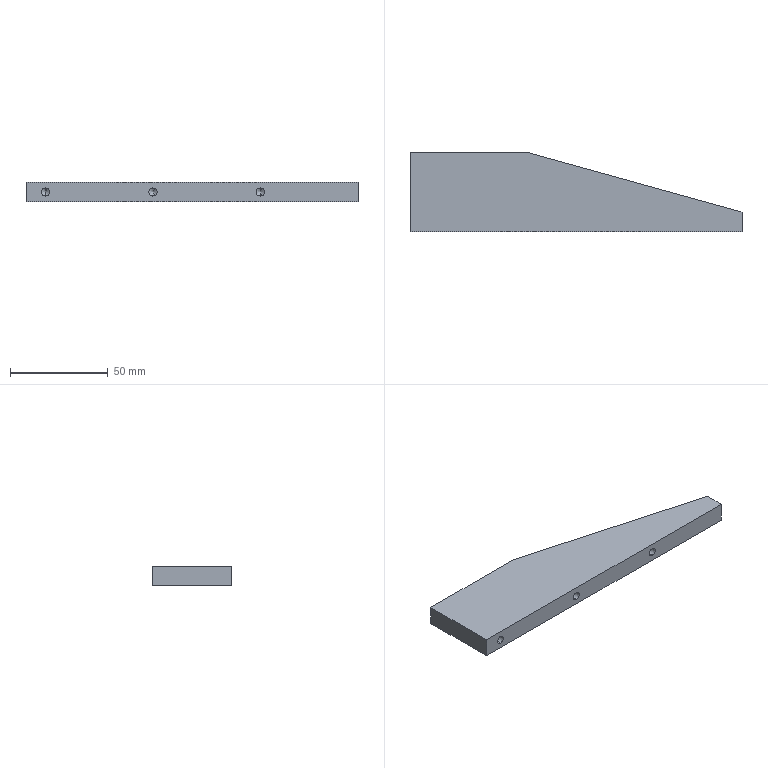Part | STEP file | PN_0090 Mount electronic clip mounting plate 5 | 1 solid | 27 faces | box 170 x 40.5 x 10 mm | volume 51076 mm3 | cylinder 10 | cone 10 | plane 7 | commonest cylinder face diameters 4.2 x10